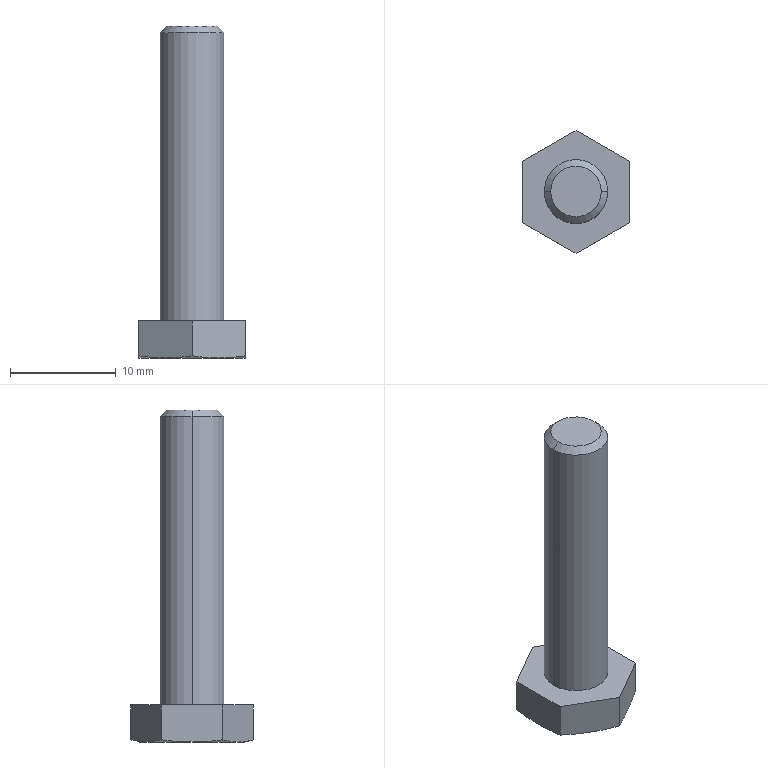Part | SolidWorks | features RefAxis 3, 3DProfileFeature 1, ICE 1, Revolution 1 | 1 solid | 19 faces | box 10.046 x 11.6 x 31.333 mm | volume 1089 mm3 | plane 9 | cone 8 | cylinder 2 | commonest cylinder face diameters 6 x2
STEP:
#1=CARTESIAN_POINT('',(3.,0.,-18.5));
#2=VERTEX_POINT('',#1);
#3=CARTESIAN_POINT('',(-3.,0.,-18.5));
#4=VERTEX_POINT('',#3);
#5=CARTESIAN_POINT('',(0.,0.,-18.5));
#6=DIRECTION('',(0.,0.,1.));
#7=DIRECTION('',(1.,0.,0.));
#8=AXIS2_PLACEMENT_3D('',#5,#6,#7);
#9=CIRCLE('',#8,3.);
#10=EDGE_CURVE('',#2,#4,#9,.T.);
#11=ORIENTED_EDGE('',*,*,#10,.T.);
#12=CARTESIAN_POINT('',(-3.,0.,8.72));
#13=VERTEX_POINT('',#12);
#14=CARTESIAN_POINT('',(-3.,0.,-22.));
#15=DIRECTION('',(0.,0.,1.));
#16=VECTOR('',#15,1000.);
#17=LINE('',#14,#16);
#18=EDGE_CURVE('',#4,#13,#17,.T.);
#19=ORIENTED_EDGE('',*,*,#18,.T.);
#20=CARTESIAN_POINT('',(3.,0.,8.72));
#21=VERTEX_POINT('',#20);
#22=CARTESIAN_POINT('',(0.,0.,8.72));
#23=DIRECTION('',(0.,0.,1.));
#24=DIRECTION('',(1.,0.,0.));
#25=AXIS2_PLACEMENT_3D('',#22,#23,#24);
#26=CIRCLE('',#25,3.);
#27=EDGE_CURVE('',#21,#13,#26,.T.);
#28=ORIENTED_EDGE('',*,*,#27,.F.);
#29=CARTESIAN_POINT('',(3.,0.,-22.));
#30=DIRECTION('',(0.,0.,1.));
#31=VECTOR('',#30,1000.);
#32=LINE('',#29,#31);
#33=EDGE_CURVE('',#2,#21,#32,.T.);
#34=ORIENTED_EDGE('',*,*,#33,.F.);
#35=EDGE_LOOP('',(#11,#19,#28,#34));
#36=FACE_OUTER_BOUND('',#35,.T.);
#37=CARTESIAN_POINT('',(0.,0.,-22.));
#38=DIRECTION('',(0.,0.,1.));
#39=DIRECTION('',(1.,0.,0.));
#40=AXIS2_PLACEMENT_3D('',#37,#38,#39);
#41=CYLINDRICAL_SURFACE('',#40,3.);
#42=ADVANCED_FACE('',(#36),#41,.T.);
#43=CARTESIAN_POINT('',(2.386,0.,9.333));
#44=VERTEX_POINT('',#43);
#45=CARTESIAN_POINT('',(-2.386,0.,9.333));
#46=VERTEX_POINT('',#45);
#47=CARTESIAN_POINT('',(0.,0.,9.333));
#48=DIRECTION('',(0.,0.,1.));
#49=DIRECTION('',(1.,0.,0.));
#50=AXIS2_PLACEMENT_3D('',#47,#48,#49);
#51=CIRCLE('',#50,2.386);
#52=EDGE_CURVE('',#44,#46,#51,.T.);
#53=ORIENTED_EDGE('',*,*,#52,.F.);
#54=CARTESIAN_POINT('',(3.,0.,8.72));
#55=DIRECTION('',(0.7071,0.,-0.7071));
#56=VECTOR('',#55,1000.);
#57=LINE('',#54,#56);
#58=EDGE_CURVE('',#44,#21,#57,.T.);
#59=ORIENTED_EDGE('',*,*,#58,.T.);
#60=ORIENTED_EDGE('',*,*,#27,.T.);
#61=CARTESIAN_POINT('',(-3.,0.,8.72));
#62=DIRECTION('',(-0.7071,0.,-0.7071));
#63=VECTOR('',#62,1000.);
#64=LINE('',#61,#63);
#65=EDGE_CURVE('',#46,#13,#64,.T.);
#66=ORIENTED_EDGE('',*,*,#65,.F.);
#67=EDGE_LOOP('',(#53,#59,#60,#66));
#68=FACE_OUTER_BOUND('',#67,.T.);
#69=CARTESIAN_POINT('',(0.,0.,8.72));
#70=DIRECTION('',(0.,0.,-1.));
#71=DIRECTION('',(-1.,0.,0.));
#72=AXIS2_PLACEMENT_3D('',#69,#70,#71);
#73=CONICAL_SURFACE('',#72,3.,0.7854);
#74=ADVANCED_FACE('',(#68),#73,.T.);
#75=ORIENTED_EDGE('',*,*,#10,.F.);
#76=CARTESIAN_POINT('',(0.,0.,-18.5));
#77=DIRECTION('',(0.,0.,1.));
#78=DIRECTION('',(1.,0.,0.));
#79=AXIS2_PLACEMENT_3D('',#76,#77,#78);
#80=CIRCLE('',#79,3.);
#81=EDGE_CURVE('',#4,#2,#80,.T.);
#82=ORIENTED_EDGE('',*,*,#81,.F.);
#83=EDGE_LOOP('',(#75,#82));
#84=FACE_BOUND('',#83,.T.);
#85=CARTESIAN_POINT('',(5.023,-2.9,-18.5));
#86=VERTEX_POINT('',#85);
#87=CARTESIAN_POINT('',(0.,-5.8,-18.5));
#88=VERTEX_POINT('',#87);
#89=CARTESIAN_POINT('',(5.023,-2.9,-18.5));
#90=DIRECTION('',(-0.866,-0.5,0.));
#91=VECTOR('',#90,1000.);
#92=LINE('',#89,#91);
#93=EDGE_CURVE('',#86,#88,#92,.T.);
#94=ORIENTED_EDGE('',*,*,#93,.F.);
#95=CARTESIAN_POINT('',(5.023,2.9,-18.5));
#96=VERTEX_POINT('',#95);
#97=CARTESIAN_POINT('',(5.023,2.9,-18.5));
#98=DIRECTION('',(0.,-1.,0.));
#99=VECTOR('',#98,1000.);
#100=LINE('',#97,#99);
#101=EDGE_CURVE('',#96,#86,#100,.T.);
#102=ORIENTED_EDGE('',*,*,#101,.F.);
#103=CARTESIAN_POINT('',(0.,5.8,-18.5));
#104=VERTEX_POINT('',#103);
#105=CARTESIAN_POINT('',(0.,5.8,-18.5));
#106=DIRECTION('',(0.866,-0.5,0.));
#107=VECTOR('',#106,1000.);
#108=LINE('',#105,#107);
#109=EDGE_CURVE('',#104,#96,#108,.T.);
#110=ORIENTED_EDGE('',*,*,#109,.F.);
#111=CARTESIAN_POINT('',(-5.023,2.9,-18.5));
#112=VERTEX_POINT('',#111);
#113=CARTESIAN_POINT('',(-5.023,2.9,-18.5));
#114=DIRECTION('',(0.866,0.5,0.));
#115=VECTOR('',#114,1000.);
#116=LINE('',#113,#115);
#117=EDGE_CURVE('',#112,#104,#116,.T.);
#118=ORIENTED_EDGE('',*,*,#117,.F.);
#119=CARTESIAN_POINT('',(-5.023,-2.9,-18.5));
#120=VERTEX_POINT('',#119);
#121=CARTESIAN_POINT('',(-5.023,-2.9,-18.5));
#122=DIRECTION('',(0.,1.,0.));
#123=VECTOR('',#122,1000.);
#124=LINE('',#121,#123);
#125=EDGE_CURVE('',#120,#112,#124,.T.);
#126=ORIENTED_EDGE('',*,*,#125,.F.);
#127=CARTESIAN_POINT('',(0.,-5.8,-18.5));
#128=DIRECTION('',(-0.866,0.5,0.));
#129=VECTOR('',#128,1000.);
#130=LINE('',#127,#129);
#131=EDGE_CURVE('',#88,#120,#130,.T.);
#132=ORIENTED_EDGE('',*,*,#131,.F.);
#133=EDGE_LOOP('',(#94,#102,#110,#118,#126,#132));
#134=FACE_OUTER_BOUND('',#133,.T.);
#135=CARTESIAN_POINT('',(0.,3.,-18.5));
#136=DIRECTION('',(0.,0.,-1.));
#137=DIRECTION('',(-1.,0.,0.));
#138=AXIS2_PLACEMENT_3D('',#135,#136,#137);
#139=PLANE('',#138);
#140=ADVANCED_FACE('',(#84,#134),#139,.F.);
#141=CARTESIAN_POINT('',(0.,0.,9.333));
#142=DIRECTION('',(0.,0.,1.));
#143=DIRECTION('',(1.,0.,0.));
#144=AXIS2_PLACEMENT_3D('',#141,#142,#143);
#145=CIRCLE('',#144,2.386);
#146=EDGE_CURVE('',#46,#44,#145,.T.);
#147=ORIENTED_EDGE('',*,*,#146,.T.);
#148=ORIENTED_EDGE('',*,*,#52,.T.);
#149=EDGE_LOOP('',(#147,#148));
#150=FACE_OUTER_BOUND('',#149,.T.);
#151=CARTESIAN_POINT('',(0.,0.,9.333));
#152=DIRECTION('',(0.,0.,-1.));
#153=DIRECTION('',(-1.,0.,0.));
#154=AXIS2_PLACEMENT_3D('',#151,#152,#153);
#155=PLANE('',#154);
#156=ADVANCED_FACE('',(#150),#155,.F.);
#157=ORIENTED_EDGE('',*,*,#58,.F.);
#158=ORIENTED_EDGE('',*,*,#146,.F.);
#159=ORIENTED_EDGE('',*,*,#65,.T.);
#160=CARTESIAN_POINT('',(0.,0.,8.72));
#161=DIRECTION('',(0.,0.,1.));
#162=DIRECTION('',(1.,0.,0.));
#163=AXIS2_PLACEMENT_3D('',#160,#161,#162);
#164=CIRCLE('',#163,3.);
#165=EDGE_CURVE('',#13,#21,#164,.T.);
#166=ORIENTED_EDGE('',*,*,#165,.T.);
#167=EDGE_LOOP('',(#157,#158,#159,#166));
#168=FACE_OUTER_BOUND('',#167,.T.);
#169=CARTESIAN_POINT('',(0.,0.,8.72));
#170=DIRECTION('',(0.,0.,-1.));
#171=DIRECTION('',(-1.,0.,0.));
#172=AXIS2_PLACEMENT_3D('',#169,#170,#171);
#173=CONICAL_SURFACE('',#172,3.,0.7854);
#174=ADVANCED_FACE('',(#168),#173,.T.);
#175=ORIENTED_EDGE('',*,*,#18,.F.);
#176=ORIENTED_EDGE('',*,*,#81,.T.);
#177=ORIENTED_EDGE('',*,*,#33,.T.);
#178=ORIENTED_EDGE('',*,*,#165,.F.);
#179=EDGE_LOOP('',(#175,#176,#177,#178));
#180=FACE_OUTER_BOUND('',#179,.T.);
#181=CARTESIAN_POINT('',(0.,0.,-22.));
#182=DIRECTION('',(0.,0.,1.));
#183=DIRECTION('',(1.,0.,0.));
#184=AXIS2_PLACEMENT_3D('',#181,#182,#183);
#185=CYLINDRICAL_SURFACE('',#184,3.);
#186=ADVANCED_FACE('',(#180),#185,.T.);
#187=CARTESIAN_POINT('',(0.,-5.8,-21.792));
#188=VERTEX_POINT('',#187);
#189=CARTESIAN_POINT('',(2.511,-4.35,-22.));
#190=VERTEX_POINT('',#189);
#191=CARTESIAN_POINT('',(0.,-5.8,-21.792));
#192=CARTESIAN_POINT('',(0.8372,-5.317,-21.921));
#193=CARTESIAN_POINT('',(1.674,-4.833,-22.));
#194=CARTESIAN_POINT('',(2.511,-4.35,-22.));
#195=B_SPLINE_CURVE_WITH_KNOTS('',3,(#191,#192,#193,#194),.UNSPECIFIED.,.F.,.F.,(4,4),(0.000000231,0.0029),.UNSPECIFIED.);
#196=EDGE_CURVE('',#188,#190,#195,.T.);
#197=ORIENTED_EDGE('',*,*,#196,.T.);
#198=CARTESIAN_POINT('',(5.023,-2.9,-21.792));
#199=VERTEX_POINT('',#198);
#200=CARTESIAN_POINT('',(2.511,-4.35,-22.));
#201=CARTESIAN_POINT('',(3.349,-3.867,-22.));
#202=CARTESIAN_POINT('',(4.186,-3.383,-21.921));
#203=CARTESIAN_POINT('',(5.023,-2.9,-21.792));
#204=B_SPLINE_CURVE_WITH_KNOTS('',3,(#200,#201,#202,#203),.UNSPECIFIED.,.F.,.F.,(4,4),(0.0029,0.0058),.UNSPECIFIED.);
#205=EDGE_CURVE('',#190,#199,#204,.T.);
#206=ORIENTED_EDGE('',*,*,#205,.T.);
#207=CARTESIAN_POINT('',(5.023,-2.9,-18.5));
#208=DIRECTION('',(0.,0.,-1.));
#209=VECTOR('',#208,1000.);
#210=LINE('',#207,#209);
#211=EDGE_CURVE('',#86,#199,#210,.T.);
#212=ORIENTED_EDGE('',*,*,#211,.F.);
#213=ORIENTED_EDGE('',*,*,#93,.T.);
#214=CARTESIAN_POINT('',(0.,-5.8,-18.5));
#215=DIRECTION('',(0.,0.,-1.));
#216=VECTOR('',#215,1000.);
#217=LINE('',#214,#216);
#218=EDGE_CURVE('',#88,#188,#217,.T.);
#219=ORIENTED_EDGE('',*,*,#218,.T.);
#220=EDGE_LOOP('',(#197,#206,#212,#213,#219));
#221=FACE_OUTER_BOUND('',#220,.T.);
#222=CARTESIAN_POINT('',(5.023,-2.9,-18.5));
#223=DIRECTION('',(0.5,-0.866,0.));
#224=DIRECTION('',(0.866,0.5,0.));
#225=AXIS2_PLACEMENT_3D('',#222,#223,#224);
#226=PLANE('',#225);
#227=ADVANCED_FACE('',(#221),#226,.T.);
#228=CARTESIAN_POINT('',(5.023,0.,-22.));
#229=VERTEX_POINT('',#228);
#230=CARTESIAN_POINT('',(5.023,-2.9,-21.792));
#231=CARTESIAN_POINT('',(5.023,-2.418,-21.856));
#232=CARTESIAN_POINT('',(5.023,-1.933,-21.909));
#233=CARTESIAN_POINT('',(5.023,-0.9659,-21.981));
#234=CARTESIAN_POINT('',(5.023,-0.4827,-22.));
#235=CARTESIAN_POINT('',(5.023,0.,-22.));
#236=B_SPLINE_CURVE_WITH_KNOTS('',3,(#230,#231,#232,#233,#234,#235),.UNSPECIFIED.,.F.,.F.,(4,2,4),(0.004852,0.006308,0.007765),.UNSPECIFIED.);
#237=EDGE_CURVE('',#199,#229,#236,.T.);
#238=ORIENTED_EDGE('',*,*,#237,.T.);
#239=CARTESIAN_POINT('',(5.023,2.9,-21.792));
#240=VERTEX_POINT('',#239);
#241=CARTESIAN_POINT('',(5.023,0.,-22.));
#242=CARTESIAN_POINT('',(5.023,0.9687,-22.));
#243=CARTESIAN_POINT('',(5.023,1.935,-21.921));
#244=CARTESIAN_POINT('',(5.023,2.9,-21.792));
#245=B_SPLINE_CURVE_WITH_KNOTS('',3,(#241,#242,#243,#244),.UNSPECIFIED.,.F.,.F.,(4,4),(0.007765,0.01069),.UNSPECIFIED.);
#246=EDGE_CURVE('',#229,#240,#245,.T.);
#247=ORIENTED_EDGE('',*,*,#246,.T.);
#248=CARTESIAN_POINT('',(5.023,2.9,-18.5));
#249=DIRECTION('',(0.,0.,-1.));
#250=VECTOR('',#249,1000.);
#251=LINE('',#248,#250);
#252=EDGE_CURVE('',#96,#240,#251,.T.);
#253=ORIENTED_EDGE('',*,*,#252,.F.);
#254=ORIENTED_EDGE('',*,*,#101,.T.);
#255=ORIENTED_EDGE('',*,*,#211,.T.);
#256=EDGE_LOOP('',(#238,#247,#253,#254,#255));
#257=FACE_OUTER_BOUND('',#256,.T.);
#258=CARTESIAN_POINT('',(5.023,2.9,-18.5));
#259=DIRECTION('',(1.,0.,0.));
#260=DIRECTION('',(0.,0.,-1.));
#261=AXIS2_PLACEMENT_3D('',#258,#259,#260);
#262=PLANE('',#261);
#263=ADVANCED_FACE('',(#257),#262,.T.);
#264=CARTESIAN_POINT('',(2.511,4.35,-22.));
#265=VERTEX_POINT('',#264);
#266=CARTESIAN_POINT('',(5.023,2.9,-21.792));
#267=CARTESIAN_POINT('',(4.186,3.383,-21.921));
#268=CARTESIAN_POINT('',(3.349,3.867,-22.));
#269=CARTESIAN_POINT('',(2.511,4.35,-22.));
#270=B_SPLINE_CURVE_WITH_KNOTS('',3,(#266,#267,#268,#269),.UNSPECIFIED.,.F.,.F.,(4,4),(0.000000231,0.0029),.UNSPECIFIED.);
#271=EDGE_CURVE('',#240,#265,#270,.T.);
#272=ORIENTED_EDGE('',*,*,#271,.T.);
#273=CARTESIAN_POINT('',(0.,5.8,-21.792));
#274=VERTEX_POINT('',#273);
#275=CARTESIAN_POINT('',(2.511,4.35,-22.));
#276=CARTESIAN_POINT('',(1.674,4.833,-22.));
#277=CARTESIAN_POINT('',(0.8372,5.317,-21.921));
#278=CARTESIAN_POINT('',(0.,5.8,-21.792));
#279=B_SPLINE_CURVE_WITH_KNOTS('',3,(#275,#276,#277,#278),.UNSPECIFIED.,.F.,.F.,(4,4),(0.0029,0.0058),.UNSPECIFIED.);
#280=EDGE_CURVE('',#265,#274,#279,.T.);
#281=ORIENTED_EDGE('',*,*,#280,.T.);
#282=CARTESIAN_POINT('',(0.,5.8,-18.5));
#283=DIRECTION('',(0.,0.,-1.));
#284=VECTOR('',#283,1000.);
#285=LINE('',#282,#284);
#286=EDGE_CURVE('',#104,#274,#285,.T.);
#287=ORIENTED_EDGE('',*,*,#286,.F.);
#288=ORIENTED_EDGE('',*,*,#109,.T.);
#289=ORIENTED_EDGE('',*,*,#252,.T.);
#290=EDGE_LOOP('',(#272,#281,#287,#288,#289));
#291=FACE_OUTER_BOUND('',#290,.T.);
#292=CARTESIAN_POINT('',(0.,5.8,-18.5));
#293=DIRECTION('',(0.5,0.866,0.));
#294=DIRECTION('',(-0.866,0.5,0.));
#295=AXIS2_PLACEMENT_3D('',#292,#293,#294);
#296=PLANE('',#295);
#297=ADVANCED_FACE('',(#291),#296,.T.);
#298=CARTESIAN_POINT('',(-2.511,4.35,-22.));
#299=VERTEX_POINT('',#298);
#300=CARTESIAN_POINT('',(0.,5.8,-21.792));
#301=CARTESIAN_POINT('',(-0.8372,5.317,-21.921));
#302=CARTESIAN_POINT('',(-1.674,4.833,-22.));
#303=CARTESIAN_POINT('',(-2.511,4.35,-22.));
#304=B_SPLINE_CURVE_WITH_KNOTS('',3,(#300,#301,#302,#303),.UNSPECIFIED.,.F.,.F.,(4,4),(0.000000231,0.0029),.UNSPECIFIED.);
#305=EDGE_CURVE('',#274,#299,#304,.T.);
#306=ORIENTED_EDGE('',*,*,#305,.T.);
#307=CARTESIAN_POINT('',(-5.023,2.9,-21.792));
#308=VERTEX_POINT('',#307);
#309=CARTESIAN_POINT('',(-2.511,4.35,-22.));
#310=CARTESIAN_POINT('',(-3.349,3.867,-22.));
#311=CARTESIAN_POINT('',(-4.186,3.383,-21.921));
#312=CARTESIAN_POINT('',(-5.023,2.9,-21.792));
#313=B_SPLINE_CURVE_WITH_KNOTS('',3,(#309,#310,#311,#312),.UNSPECIFIED.,.F.,.F.,(4,4),(0.0029,0.0058),.UNSPECIFIED.);
#314=EDGE_CURVE('',#299,#308,#313,.T.);
#315=ORIENTED_EDGE('',*,*,#314,.T.);
#316=CARTESIAN_POINT('',(-5.023,2.9,-18.5));
#317=DIRECTION('',(0.,0.,-1.));
#318=VECTOR('',#317,1000.);
#319=LINE('',#316,#318);
#320=EDGE_CURVE('',#112,#308,#319,.T.);
#321=ORIENTED_EDGE('',*,*,#320,.F.);
#322=ORIENTED_EDGE('',*,*,#117,.T.);
#323=ORIENTED_EDGE('',*,*,#286,.T.);
#324=EDGE_LOOP('',(#306,#315,#321,#322,#323));
#325=FACE_OUTER_BOUND('',#324,.T.);
#326=CARTESIAN_POINT('',(-5.023,2.9,-18.5));
#327=DIRECTION('',(-0.5,0.866,0.));
#328=DIRECTION('',(-0.866,-0.5,0.));
#329=AXIS2_PLACEMENT_3D('',#326,#327,#328);
#330=PLANE('',#329);
#331=ADVANCED_FACE('',(#325),#330,.T.);
#332=CARTESIAN_POINT('',(-5.023,0.,-22.));
#333=VERTEX_POINT('',#332);
#334=CARTESIAN_POINT('',(-5.023,2.9,-21.792));
#335=CARTESIAN_POINT('',(-5.023,1.935,-21.921));
#336=CARTESIAN_POINT('',(-5.023,0.9687,-22.));
#337=CARTESIAN_POINT('',(-5.023,0.,-22.));
#338=B_SPLINE_CURVE_WITH_KNOTS('',3,(#334,#335,#336,#337),.UNSPECIFIED.,.F.,.F.,(4,4),(0.01103,0.01395),.UNSPECIFIED.);
#339=EDGE_CURVE('',#308,#333,#338,.T.);
#340=ORIENTED_EDGE('',*,*,#339,.T.);
#341=CARTESIAN_POINT('',(-5.023,-2.9,-21.792));
#342=VERTEX_POINT('',#341);
#343=CARTESIAN_POINT('',(-5.023,0.,-22.));
#344=CARTESIAN_POINT('',(-5.023,-0.4827,-22.));
#345=CARTESIAN_POINT('',(-5.023,-0.9659,-21.981));
#346=CARTESIAN_POINT('',(-5.023,-1.933,-21.909));
#347=CARTESIAN_POINT('',(-5.023,-2.418,-21.856));
#348=CARTESIAN_POINT('',(-5.023,-2.9,-21.792));
#349=B_SPLINE_CURVE_WITH_KNOTS('',3,(#343,#344,#345,#346,#347,#348),.UNSPECIFIED.,.F.,.F.,(4,2,4),(0.01395,0.01541,0.01686),.UNSPECIFIED.);
#350=EDGE_CURVE('',#333,#342,#349,.T.);
#351=ORIENTED_EDGE('',*,*,#350,.T.);
#352=CARTESIAN_POINT('',(-5.023,-2.9,-18.5));
#353=DIRECTION('',(0.,0.,-1.));
#354=VECTOR('',#353,1000.);
#355=LINE('',#352,#354);
#356=EDGE_CURVE('',#120,#342,#355,.T.);
#357=ORIENTED_EDGE('',*,*,#356,.F.);
#358=ORIENTED_EDGE('',*,*,#125,.T.);
#359=ORIENTED_EDGE('',*,*,#320,.T.);
#360=EDGE_LOOP('',(#340,#351,#357,#358,#359));
#361=FACE_OUTER_BOUND('',#360,.T.);
#362=CARTESIAN_POINT('',(-5.023,-2.9,-18.5));
#363=DIRECTION('',(-1.,0.,0.));
#364=DIRECTION('',(0.,0.,1.));
#365=AXIS2_PLACEMENT_3D('',#362,#363,#364);
#366=PLANE('',#365);
#367=ADVANCED_FACE('',(#361),#366,.T.);
#368=CARTESIAN_POINT('',(-2.511,-4.35,-22.));
#369=VERTEX_POINT('',#368);
#370=CARTESIAN_POINT('',(-5.023,-2.9,-21.792));
#371=CARTESIAN_POINT('',(-4.186,-3.383,-21.921));
#372=CARTESIAN_POINT('',(-3.349,-3.867,-22.));
#373=CARTESIAN_POINT('',(-2.511,-4.35,-22.));
#374=B_SPLINE_CURVE_WITH_KNOTS('',3,(#370,#371,#372,#373),.UNSPECIFIED.,.F.,.F.,(4,4),(0.000000231,0.0029),.UNSPECIFIED.);
#375=EDGE_CURVE('',#342,#369,#374,.T.);
#376=ORIENTED_EDGE('',*,*,#375,.T.);
#377=CARTESIAN_POINT('',(-2.511,-4.35,-22.));
#378=CARTESIAN_POINT('',(-1.674,-4.833,-22.));
#379=CARTESIAN_POINT('',(-0.8372,-5.317,-21.921));
#380=CARTESIAN_POINT('',(0.,-5.8,-21.792));
#381=B_SPLINE_CURVE_WITH_KNOTS('',3,(#377,#378,#379,#380),.UNSPECIFIED.,.F.,.F.,(4,4),(0.0029,0.0058),.UNSPECIFIED.);
#382=EDGE_CURVE('',#369,#188,#381,.T.);
#383=ORIENTED_EDGE('',*,*,#382,.T.);
#384=ORIENTED_EDGE('',*,*,#218,.F.);
#385=ORIENTED_EDGE('',*,*,#131,.T.);
#386=ORIENTED_EDGE('',*,*,#356,.T.);
#387=EDGE_LOOP('',(#376,#383,#384,#385,#386));
#388=FACE_OUTER_BOUND('',#387,.T.);
#389=CARTESIAN_POINT('',(0.,-5.8,-18.5));
#390=DIRECTION('',(-0.5,-0.866,0.));
#391=DIRECTION('',(0.866,-0.5,0.));
#392=AXIS2_PLACEMENT_3D('',#389,#390,#391);
#393=PLANE('',#392);
#394=ADVANCED_FACE('',(#388),#393,.T.);
#395=ORIENTED_EDGE('',*,*,#280,.F.);
#396=CARTESIAN_POINT('',(0.,0.,-22.));
#397=DIRECTION('',(0.,0.,1.));
#398=DIRECTION('',(1.,0.,0.));
#399=AXIS2_PLACEMENT_3D('',#396,#397,#398);
#400=CIRCLE('',#399,5.023);
#401=EDGE_CURVE('',#265,#299,#400,.T.);
#402=ORIENTED_EDGE('',*,*,#401,.T.);
#403=ORIENTED_EDGE('',*,*,#305,.F.);
#404=EDGE_LOOP('',(#395,#402,#403));
#405=FACE_OUTER_BOUND('',#404,.T.);
#406=CARTESIAN_POINT('',(0.,0.,-22.));
#407=DIRECTION('',(0.,0.,1.));
#408=DIRECTION('',(1.,0.,0.));
#409=AXIS2_PLACEMENT_3D('',#406,#407,#408);
#410=CONICAL_SURFACE('',#409,5.023,1.309);
#411=ADVANCED_FACE('',(#405),#410,.T.);
#412=ORIENTED_EDGE('',*,*,#314,.F.);
#413=CARTESIAN_POINT('',(0.,0.,-22.));
#414=DIRECTION('',(0.,0.,1.));
#415=DIRECTION('',(1.,0.,0.));
#416=AXIS2_PLACEMENT_3D('',#413,#414,#415);
#417=CIRCLE('',#416,5.023);
#418=EDGE_CURVE('',#299,#333,#417,.T.);
#419=ORIENTED_EDGE('',*,*,#418,.T.);
#420=ORIENTED_EDGE('',*,*,#339,.F.);
#421=EDGE_LOOP('',(#412,#419,#420));
#422=FACE_OUTER_BOUND('',#421,.T.);
#423=CARTESIAN_POINT('',(0.,0.,-22.));
#424=DIRECTION('',(0.,0.,1.));
#425=DIRECTION('',(1.,0.,0.));
#426=AXIS2_PLACEMENT_3D('',#423,#424,#425);
#427=CONICAL_SURFACE('',#426,5.023,1.309);
#428=ADVANCED_FACE('',(#422),#427,.T.);
#429=ORIENTED_EDGE('',*,*,#350,.F.);
#430=CARTESIAN_POINT('',(0.,0.,-22.));
#431=DIRECTION('',(0.,0.,1.));
#432=DIRECTION('',(1.,0.,0.));
#433=AXIS2_PLACEMENT_3D('',#430,#431,#432);
#434=CIRCLE('',#433,5.023);
#435=EDGE_CURVE('',#333,#369,#434,.T.);
#436=ORIENTED_EDGE('',*,*,#435,.T.);
#437=ORIENTED_EDGE('',*,*,#375,.F.);
#438=EDGE_LOOP('',(#429,#436,#437));
#439=FACE_OUTER_BOUND('',#438,.T.);
#440=CARTESIAN_POINT('',(0.,0.,-22.));
#441=DIRECTION('',(0.,0.,1.));
#442=DIRECTION('',(1.,0.,0.));
#443=AXIS2_PLACEMENT_3D('',#440,#441,#442);
#444=CONICAL_SURFACE('',#443,5.023,1.309);
#445=ADVANCED_FACE('',(#439),#444,.T.);
#446=ORIENTED_EDGE('',*,*,#205,.F.);
#447=CARTESIAN_POINT('',(0.,0.,-22.));
#448=DIRECTION('',(0.,0.,1.));
#449=DIRECTION('',(1.,0.,0.));
#450=AXIS2_PLACEMENT_3D('',#447,#448,#449);
#451=CIRCLE('',#450,5.023);
#452=EDGE_CURVE('',#190,#229,#451,.T.);
#453=ORIENTED_EDGE('',*,*,#452,.T.);
#454=ORIENTED_EDGE('',*,*,#237,.F.);
#455=EDGE_LOOP('',(#446,#453,#454));
#456=FACE_OUTER_BOUND('',#455,.T.);
#457=CARTESIAN_POINT('',(0.,0.,-22.));
#458=DIRECTION('',(0.,0.,1.));
#459=DIRECTION('',(1.,0.,0.));
#460=AXIS2_PLACEMENT_3D('',#457,#458,#459);
#461=CONICAL_SURFACE('',#460,5.023,1.309);
#462=ADVANCED_FACE('',(#456),#461,.T.);
#463=ORIENTED_EDGE('',*,*,#246,.F.);
#464=CARTESIAN_POINT('',(0.,0.,-22.));
#465=DIRECTION('',(0.,0.,1.));
#466=DIRECTION('',(1.,0.,0.));
#467=AXIS2_PLACEMENT_3D('',#464,#465,#466);
#468=CIRCLE('',#467,5.023);
#469=EDGE_CURVE('',#229,#265,#468,.T.);
#470=ORIENTED_EDGE('',*,*,#469,.T.);
#471=ORIENTED_EDGE('',*,*,#271,.F.);
#472=EDGE_LOOP('',(#463,#470,#471));
#473=FACE_OUTER_BOUND('',#472,.T.);
#474=CARTESIAN_POINT('',(0.,0.,-22.));
#475=DIRECTION('',(0.,0.,1.));
#476=DIRECTION('',(1.,0.,0.));
#477=AXIS2_PLACEMENT_3D('',#474,#475,#476);
#478=CONICAL_SURFACE('',#477,5.023,1.309);
#479=ADVANCED_FACE('',(#473),#478,.T.);
#480=ORIENTED_EDGE('',*,*,#469,.F.);
#481=ORIENTED_EDGE('',*,*,#452,.F.);
#482=CARTESIAN_POINT('',(0.,0.,-22.));
#483=DIRECTION('',(0.,0.,1.));
#484=DIRECTION('',(1.,0.,0.));
#485=AXIS2_PLACEMENT_3D('',#482,#483,#484);
#486=CIRCLE('',#485,5.023);
#487=EDGE_CURVE('',#369,#190,#486,.T.);
#488=ORIENTED_EDGE('',*,*,#487,.F.);
#489=ORIENTED_EDGE('',*,*,#435,.F.);
#490=ORIENTED_EDGE('',*,*,#418,.F.);
#491=ORIENTED_EDGE('',*,*,#401,.F.);
#492=EDGE_LOOP('',(#480,#481,#488,#489,#490,#491));
#493=FACE_OUTER_BOUND('',#492,.T.);
#494=CARTESIAN_POINT('',(0.,5.023,-22.));
#495=DIRECTION('',(0.,0.,1.));
#496=DIRECTION('',(1.,0.,0.));
#497=AXIS2_PLACEMENT_3D('',#494,#495,#496);
#498=PLANE('',#497);
#499=ADVANCED_FACE('',(#493),#498,.F.);
#500=ORIENTED_EDGE('',*,*,#196,.F.);
#501=ORIENTED_EDGE('',*,*,#382,.F.);
#502=ORIENTED_EDGE('',*,*,#487,.T.);
#503=EDGE_LOOP('',(#500,#501,#502));
#504=FACE_OUTER_BOUND('',#503,.T.);
#505=CARTESIAN_POINT('',(0.,0.,-22.));
#506=DIRECTION('',(0.,0.,1.));
#507=DIRECTION('',(1.,0.,0.));
#508=AXIS2_PLACEMENT_3D('',#505,#506,#507);
#509=CONICAL_SURFACE('',#508,5.023,1.309);
#510=ADVANCED_FACE('',(#504),#509,.T.);
#511=CLOSED_SHELL('',(#42,#74,#140,#156,#174,#186,#227,#263,#297,#331,#367,#394,#411,#428,#445,#462,#479,#499,#510));
#512=MANIFOLD_SOLID_BREP('',#511);
#513=CARTESIAN_POINT('',(0.,0.,0.));
#514=DIRECTION('',(0.,0.,1.));
#515=DIRECTION('',(1.,0.,0.));
#516=AXIS2_PLACEMENT_3D('',#513,#514,#515);
#517=(LENGTH_UNIT()NAMED_UNIT(*)SI_UNIT(.MILLI.,.METRE.));
#518=UNCERTAINTY_MEASURE_WITH_UNIT(LENGTH_MEASURE(0.00001),#517,'','');
#519=(NAMED_UNIT(*)PLANE_ANGLE_UNIT()SI_UNIT($,.RADIAN.));
#520=(NAMED_UNIT(*)SI_UNIT($,.STERADIAN.)SOLID_ANGLE_UNIT());
#521=(GEOMETRIC_REPRESENTATION_CONTEXT(3)GLOBAL_UNCERTAINTY_ASSIGNED_CONTEXT((#518))GLOBAL_UNIT_ASSIGNED_CONTEXT((#517,#519,#520))REPRESENTATION_CONTEXT('',''));
#522=ADVANCED_BREP_SHAPE_REPRESENTATION('',(#512,#516),#521);